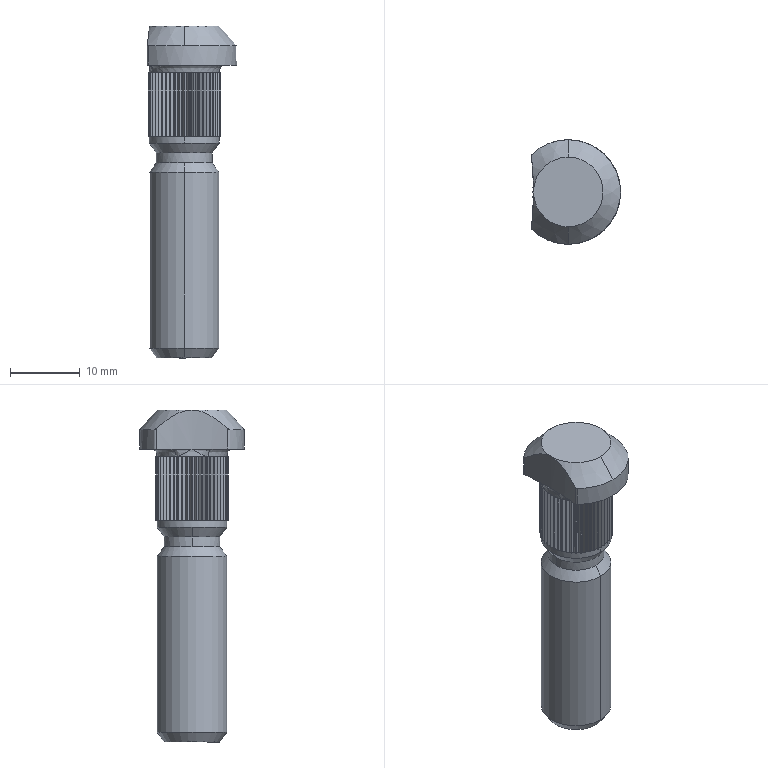Part | SolidWorks | features ICE 6, Chamfer 2, Fillet 2, Extrusion 1, Scale 1 | 1 solid | 413 faces | box 12.785 x 15 x 47.6 mm | volume 3973 mm3 | plane 339 | cylinder 61 | cone 9 | spline 4 | commonest cylinder face diameters 9.6 x48 10 x6 0.8 x3 8 x2 15 x1 92.5 x1